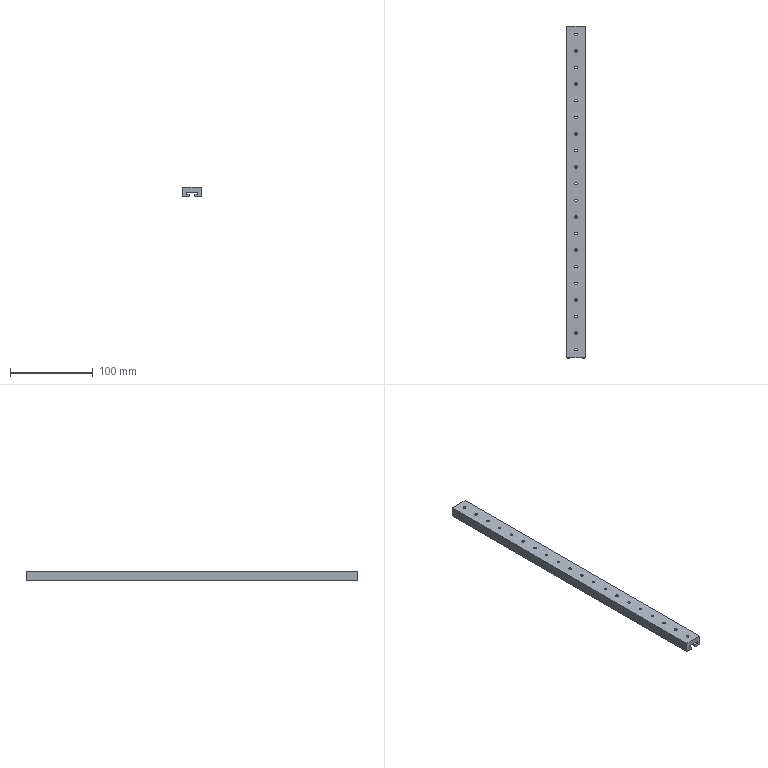Part | SolidWorks | features BaseBody 1 | 1 solid | 158 faces | box 22 x 400 x 12 mm | volume 79544 mm3 | cylinder 80 | cone 40 | plane 38 | commonest cylinder face diameters 3.1 x40 5.7 x40